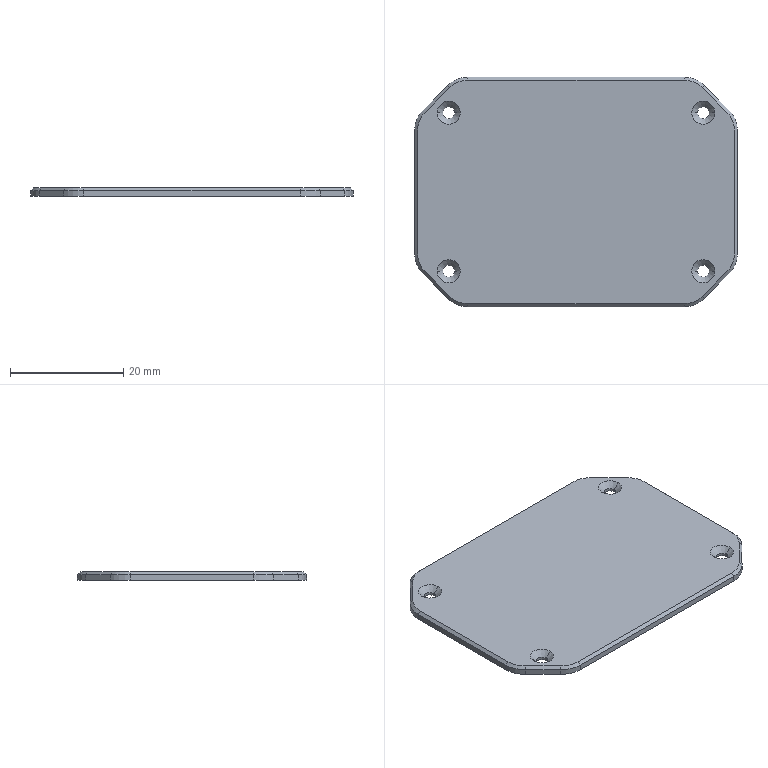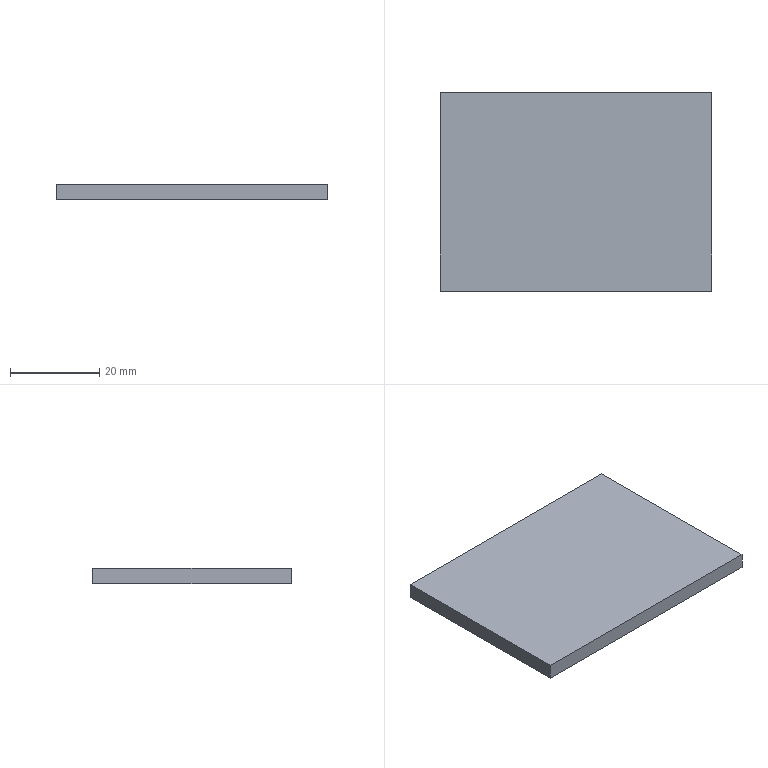CAM job | NX | 3-axis milling, drilling | part box 57 x 40.5 x 1.5 mm | stock box 61 x 44.5 x 3.5 mm
Tools:
number,name,description,diameter,corner_radius,flute_length,length,flutes
1,D4,,4.0,0.0,12.0,50.0,2
2,D3倒角,,3.0,0.0,6.0,75.0,2
4,D2.2钻头,,2.2,0.0,50.0,75.0,2
3,D3,,3.0,0.0,50.0,75.0,2
5,R0.5,,1.0,0.5,50.0,75.0,2
Operations:
program,operation,operation_type,tool,method,geometry_group,spindle_rpm,surface_speed,feed_per_tooth,feed_cut,feed_plunge,cut_length_mm,path_length_mm,cut_time_min,machine_time_min
A1,PLANAR_PROFILE,PlanarMilling,D4,MILL_ROUGH,WORKPIECE,6500.0,81.0,0.1538,2000.0,60.0,2093.845,2442.711,1.429,1.464
A1,PLANAR_PROFILE_COPY,PlanarMilling,D4,MILL_FINISH,WORKPIECE,6500.0,81.0,0.0615,800.0,100.0,195.172,232.172,0.244,0.2477
A1,PLANAR_PROFILE_COPY_COPY,PlanarMilling,D3倒角,MILL_FINISH,WORKPIECE,4500.0,42.0,0.0889,800.0,100.0,192.344,228.344,0.2404,0.244
A1,PLANAR_PROFILE_COPY_1,PlanarMilling,D4,MILL_ROUGH,WORKPIECE,6500.0,81.0,0.1538,2000.0,60.0,2093.845,2442.711,1.429,1.464
A1,PLANAR_PROFILE_COPY_COPY_1,PlanarMilling,D4,MILL_FINISH,WORKPIECE,6500.0,81.0,0.0615,800.0,100.0,195.172,232.172,0.244,0.2477
A1,PLANAR_PROFILE_COPY_COPY_COPY,PlanarMilling,D3倒角,MILL_FINISH,WORKPIECE,4500.0,42.0,0.0889,800.0,100.0,192.344,228.344,0.2404,0.244
A1,PLANAR_PROFILE_COPY_2,PlanarMilling,D4,MILL_ROUGH,WORKPIECE,6500.0,81.0,0.1538,2000.0,60.0,2093.845,2442.711,1.429,1.464
A1,PLANAR_PROFILE_COPY_COPY_2,PlanarMilling,D4,MILL_FINISH,WORKPIECE,6500.0,81.0,0.0615,800.0,100.0,195.172,232.172,0.244,0.2477
A1,PLANAR_PROFILE_COPY_COPY_COPY_1,PlanarMilling,D3倒角,MILL_FINISH,WORKPIECE,4500.0,42.0,0.0889,800.0,100.0,192.344,228.344,0.2404,0.244
A1,PLANAR_PROFILE_COPY_3,PlanarMilling,D4,MILL_ROUGH,WORKPIECE,6500.0,81.0,0.1538,2000.0,60.0,2093.845,2442.711,1.429,1.464
A1,PLANAR_PROFILE_COPY_COPY_3,PlanarMilling,D4,MILL_FINISH,WORKPIECE,6500.0,81.0,0.0615,800.0,100.0,195.172,232.172,0.244,0.2477
A1,PLANAR_PROFILE_COPY_COPY_COPY_2,PlanarMilling,D3倒角,MILL_FINISH,WORKPIECE,4500.0,42.0,0.0889,800.0,100.0,192.344,228.344,0.2404,0.244
A1,PLANAR_PROFILE_COPY_4,PlanarMilling,D4,MILL_ROUGH,WORKPIECE,6500.0,81.0,0.1538,2000.0,60.0,2007.901,2366.27,1.357,1.393
A1,PLANAR_PROFILE_COPY_COPY_4,PlanarMilling,D4,MILL_FINISH,WORKPIECE,6500.0,81.0,0.0615,800.0,100.0,195.172,231.872,0.244,0.2476
A1,PLANAR_PROFILE_COPY_COPY_COPY_3,PlanarMilling,D3倒角,MILL_FINISH,WORKPIECE,4500.0,42.0,0.0889,800.0,100.0,192.344,228.344,0.2404,0.244
A1,PLANAR_PROFILE_COPY_5,PlanarMilling,D4,MILL_ROUGH,WORKPIECE,6500.0,81.0,0.1538,2000.0,60.0,2093.845,2442.711,1.429,1.464
A1,PLANAR_PROFILE_COPY_COPY_5,PlanarMilling,D4,MILL_FINISH,WORKPIECE,6500.0,81.0,0.0615,800.0,100.0,195.172,232.172,0.244,0.2477
A1,PLANAR_PROFILE_COPY_COPY_COPY_4,PlanarMilling,D3倒角,MILL_FINISH,WORKPIECE,4500.0,42.0,0.0889,800.0,100.0,192.344,228.344,0.2404,0.244
A1,PLANAR_PROFILE_COPY_1_COPY,PlanarMilling,D4,MILL_ROUGH,WORKPIECE,6500.0,81.0,0.1538,2000.0,60.0,2093.845,2442.711,1.429,1.464
A1,PLANAR_PROFILE_COPY_COPY_1_COPY,PlanarMilling,D4,MILL_FINISH,WORKPIECE,6500.0,81.0,0.0615,800.0,100.0,195.172,232.172,0.244,0.2477
A1,PLANAR_PROFILE_COPY_COPY_COPY_COPY,PlanarMilling,D3倒角,MILL_FINISH,WORKPIECE,4500.0,42.0,0.0889,800.0,100.0,192.344,228.344,0.2404,0.244
A1,PLANAR_PROFILE_COPY_2_COPY,PlanarMilling,D4,MILL_ROUGH,WORKPIECE,6500.0,81.0,0.1538,2000.0,60.0,2093.845,2442.711,1.429,1.464
A1,PLANAR_PROFILE_COPY_COPY_2_COPY,PlanarMilling,D4,MILL_FINISH,WORKPIECE,6500.0,81.0,0.0615,800.0,100.0,195.172,232.172,0.244,0.2477
A1,PLANAR_PROFILE_COPY_COPY_COPY_1_COPY,PlanarMilling,D3倒角,MILL_FINISH,WORKPIECE,4500.0,42.0,0.0889,800.0,100.0,192.344,228.344,0.2404,0.244
A1,PLANAR_PROFILE_COPY_3_COPY,PlanarMilling,D4,MILL_ROUGH,WORKPIECE,6500.0,81.0,0.1538,2000.0,60.0,2093.845,2442.711,1.429,1.464
A1,PLANAR_PROFILE_COPY_COPY_3_COPY,PlanarMilling,D4,MILL_FINISH,WORKPIECE,6500.0,81.0,0.0615,800.0,100.0,195.172,232.172,0.244,0.2477
A1,PLANAR_PROFILE_COPY_COPY_COPY_2_COPY,PlanarMilling,D3倒角,MILL_FINISH,WORKPIECE,4500.0,42.0,0.0889,800.0,100.0,192.344,228.344,0.2404,0.244
A1,PLANAR_PROFILE_COPY_4_COPY,PlanarMilling,D4,MILL_ROUGH,WORKPIECE,6500.0,81.0,0.1538,2000.0,60.0,2007.901,2366.27,1.357,1.393
A1,PLANAR_PROFILE_COPY_COPY_4_COPY,PlanarMilling,D4,MILL_FINISH,WORKPIECE,6500.0,81.0,0.0615,800.0,100.0,195.172,231.872,0.244,0.2476
A1,PLANAR_PROFILE_COPY_COPY_COPY_3_COPY,PlanarMilling,D3倒角,MILL_FINISH,WORKPIECE,4500.0,42.0,0.0889,800.0,100.0,192.344,228.344,0.2404,0.244
A1,PLANAR_PROFILE_COPY_6,PlanarMilling,D4,MILL_ROUGH,WORKPIECE,6500.0,81.0,0.1538,2000.0,60.0,2093.845,2442.711,1.429,1.464
A1,PLANAR_PROFILE_COPY_COPY_6,PlanarMilling,D4,MILL_FINISH,WORKPIECE,6500.0,81.0,0.0615,800.0,100.0,195.172,232.172,0.244,0.2477
A1,PLANAR_PROFILE_COPY_COPY_COPY_5,PlanarMilling,D3倒角,MILL_FINISH,WORKPIECE,4500.0,42.0,0.0889,800.0,100.0,192.344,228.344,0.2404,0.244
A1,PLANAR_PROFILE_COPY_1_COPY_1,PlanarMilling,D4,MILL_ROUGH,WORKPIECE,6500.0,81.0,0.1538,2000.0,60.0,2093.845,2442.711,1.429,1.464
A1,PLANAR_PROFILE_COPY_COPY_1_COPY_1,PlanarMilling,D4,MILL_FINISH,WORKPIECE,6500.0,81.0,0.0615,800.0,100.0,195.172,232.172,0.244,0.2477
A1,PLANAR_PROFILE_COPY_COPY_COPY_COPY_1,PlanarMilling,D3倒角,MILL_FINISH,WORKPIECE,4500.0,42.0,0.0889,800.0,100.0,192.344,228.344,0.2404,0.244
A1,PLANAR_PROFILE_COPY_2_COPY_1,PlanarMilling,D4,MILL_ROUGH,WORKPIECE,6500.0,81.0,0.1538,2000.0,60.0,2093.845,2442.711,1.429,1.464
A1,PLANAR_PROFILE_COPY_COPY_2_COPY_1,PlanarMilling,D4,MILL_FINISH,WORKPIECE,6500.0,81.0,0.0615,800.0,100.0,195.172,232.172,0.244,0.2477
A1,PLANAR_PROFILE_COPY_COPY_COPY_1_COPY_1,PlanarMilling,D3倒角,MILL_FINISH,WORKPIECE,4500.0,42.0,0.0889,800.0,100.0,192.344,228.344,0.2404,0.244
A1,PLANAR_PROFILE_COPY_3_COPY_1,PlanarMilling,D4,MILL_ROUGH,WORKPIECE,6500.0,81.0,0.1538,2000.0,60.0,2093.845,2442.711,1.429,1.464
A1,PLANAR_PROFILE_COPY_COPY_3_COPY_1,PlanarMilling,D4,MILL_FINISH,WORKPIECE,6500.0,81.0,0.0615,800.0,100.0,195.172,232.172,0.244,0.2477
A1,PLANAR_PROFILE_COPY_COPY_COPY_2_COPY_1,PlanarMilling,D3倒角,MILL_FINISH,WORKPIECE,4500.0,42.0,0.0889,800.0,100.0,192.344,228.344,0.2404,0.244
A1,PLANAR_PROFILE_COPY_4_COPY_1,PlanarMilling,D4,MILL_ROUGH,WORKPIECE,6500.0,81.0,0.1538,2000.0,60.0,2007.901,2366.27,1.357,1.393
A1,PLANAR_PROFILE_COPY_COPY_4_COPY_1,PlanarMilling,D4,MILL_FINISH,WORKPIECE,6500.0,81.0,0.0615,800.0,100.0,195.172,231.872,0.244,0.2476
A1,PLANAR_PROFILE_COPY_COPY_COPY_3_COPY_1,PlanarMilling,D3倒角,MILL_FINISH,WORKPIECE,4500.0,42.0,0.0889,800.0,100.0,192.344,228.344,0.2404,0.244
A1,PLANAR_PROFILE_COPY_7,PlanarMilling,D4,MILL_ROUGH,WORKPIECE,6500.0,81.0,0.1538,2000.0,60.0,2093.845,2442.711,1.429,1.464
A1,PLANAR_PROFILE_COPY_COPY_7,PlanarMilling,D4,MILL_FINISH,WORKPIECE,6500.0,81.0,0.0615,800.0,100.0,195.172,232.172,0.244,0.2477
A1,PLANAR_PROFILE_COPY_COPY_COPY_6,PlanarMilling,D3倒角,MILL_FINISH,WORKPIECE,4500.0,42.0,0.0889,800.0,100.0,192.344,228.344,0.2404,0.244
A1,PLANAR_PROFILE_COPY_1_COPY_2,PlanarMilling,D4,MILL_ROUGH,WORKPIECE,6500.0,81.0,0.1538,2000.0,60.0,2093.845,2442.711,1.429,1.464
A1,PLANAR_PROFILE_COPY_COPY_1_COPY_2,PlanarMilling,D4,MILL_FINISH,WORKPIECE,6500.0,81.0,0.0615,800.0,100.0,195.172,232.172,0.244,0.2477
A1,PLANAR_PROFILE_COPY_COPY_COPY_COPY_2,PlanarMilling,D3倒角,MILL_FINISH,WORKPIECE,4500.0,42.0,0.0889,800.0,100.0,192.344,228.344,0.2404,0.244
A1,PLANAR_PROFILE_COPY_2_COPY_2,PlanarMilling,D4,MILL_ROUGH,WORKPIECE,6500.0,81.0,0.1538,2000.0,60.0,2093.845,2442.711,1.429,1.464
A1,PLANAR_PROFILE_COPY_COPY_2_COPY_2,PlanarMilling,D4,MILL_FINISH,WORKPIECE,6500.0,81.0,0.0615,800.0,100.0,195.172,232.172,0.244,0.2477
A1,PLANAR_PROFILE_COPY_COPY_COPY_1_COPY_2,PlanarMilling,D3倒角,MILL_FINISH,WORKPIECE,4500.0,42.0,0.0889,800.0,100.0,192.344,228.344,0.2404,0.244
A1,PLANAR_PROFILE_COPY_3_COPY_2,PlanarMilling,D4,MILL_ROUGH,WORKPIECE,6500.0,81.0,0.1538,2000.0,60.0,2093.845,2442.711,1.429,1.464
A1,PLANAR_PROFILE_COPY_COPY_3_COPY_2,PlanarMilling,D4,MILL_FINISH,WORKPIECE,6500.0,81.0,0.0615,800.0,100.0,195.172,232.172,0.244,0.2477
A1,PLANAR_PROFILE_COPY_COPY_COPY_2_COPY_2,PlanarMilling,D3倒角,MILL_FINISH,WORKPIECE,4500.0,42.0,0.0889,800.0,100.0,192.344,228.344,0.2404,0.244
A1,PLANAR_PROFILE_COPY_4_COPY_2,PlanarMilling,D4,MILL_ROUGH,WORKPIECE,6500.0,81.0,0.1538,2000.0,60.0,2007.901,2366.27,1.357,1.393
A1,PLANAR_PROFILE_COPY_COPY_4_COPY_2,PlanarMilling,D4,MILL_FINISH,WORKPIECE,6500.0,81.0,0.0615,800.0,100.0,195.172,231.872,0.244,0.2476
A1,PLANAR_PROFILE_COPY_COPY_COPY_3_COPY_2,PlanarMilling,D3倒角,MILL_FINISH,WORKPIECE,4500.0,42.0,0.0889,800.0,100.0,192.344,228.344,0.2404,0.244
B1,DRILLING,Operation,D3倒角,METHOD,WORKPIECE_COPY,2000.0,18.0,0.0625,250.0,0.0,16.4,200.16,0.0656,0.084
B1,DRILLING_COPY,Operation,D2.2钻头,METHOD,WORKPIECE_COPY,2000.0,18.0,0.0625,250.0,0.0,28.0,223.36,0.112,0.1315
1.NC,HOLE_MILLING,CylinderMilling,D3,MILL_FINISH,WORKPIECE_COPY,6500.0,61.0,0.0308,400.0,100.0,38.454,283.254,0.0961,0.1206
1.NC,PLANAR_PROFILE_1,PlanarMilling,R0.5,MILL_FINISH,WORKPIECE_COPY,4500.0,14.0,0.0889,800.0,100.0,56.2,299.64,0.0703,0.0946
1.NC,PLANAR_PROFILE_1_COPY,PlanarMilling,R0.5,MILL_FINISH,WORKPIECE_COPY,4500.0,14.0,0.0889,800.0,100.0,181.141,221.341,0.2264,0.2304
C1,PLANAR_MILL,PlanarMilling,D3,METHOD,JAW,4500.0,56.0,0.0667,600.0,100.0,1288.229,1328.529,2.147,2.151
C1,PLANAR_MILL_COPY,PlanarMilling,D3,METHOD,JAW,4500.0,56.0,0.0667,600.0,100.0,1288.229,1328.529,2.147,2.151